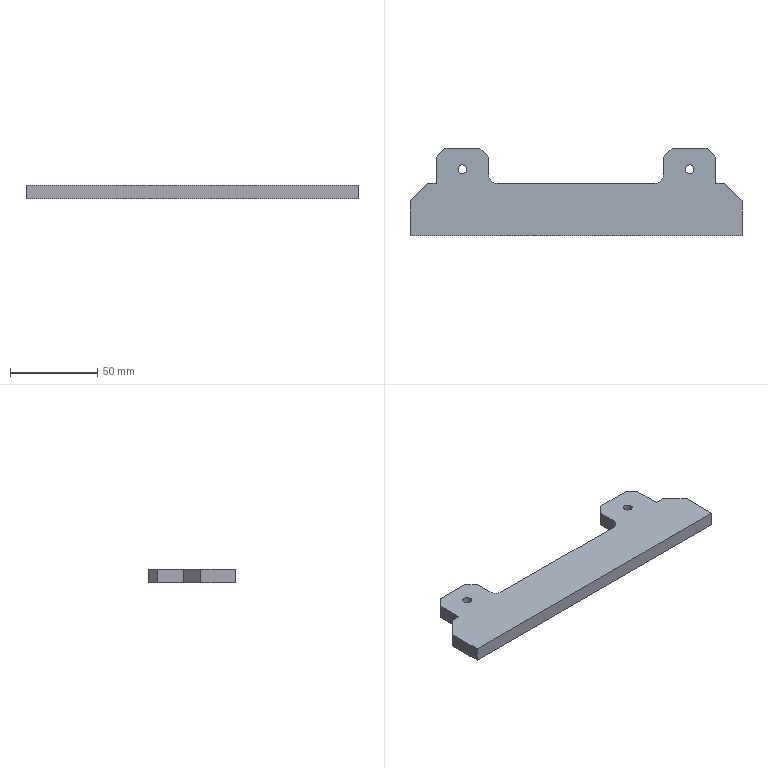Part | SolidWorks | features Chamfer 1, Extrusion 1, Fillet 1, HoleWzd 1, ICE 1 | 1 solid | 26 faces | box 190 x 50 x 8 mm | volume 53772 mm3 | plane 20 | cylinder 6 | commonest cylinder face diameters 5 x4 10 x2
STEP:
#1=CARTESIAN_POINT('',(-67.5,13.,0.));
#2=VERTEX_POINT('',#1);
#3=CARTESIAN_POINT('',(-62.5,13.,0.));
#4=VERTEX_POINT('',#3);
#5=CARTESIAN_POINT('',(-65.,13.,0.));
#6=DIRECTION('',(0.,0.,1.));
#7=DIRECTION('',(1.,0.,0.));
#8=AXIS2_PLACEMENT_3D('',#5,#6,#7);
#9=CIRCLE('',#8,2.5);
#10=EDGE_CURVE('',#2,#4,#9,.T.);
#11=ORIENTED_EDGE('',*,*,#10,.F.);
#12=CARTESIAN_POINT('',(-67.5,13.,8.));
#13=VERTEX_POINT('',#12);
#14=CARTESIAN_POINT('',(-67.5,13.,8.));
#15=DIRECTION('',(0.,0.,1.));
#16=VECTOR('',#15,1000.);
#17=LINE('',#14,#16);
#18=EDGE_CURVE('',#2,#13,#17,.T.);
#19=ORIENTED_EDGE('',*,*,#18,.T.);
#20=CARTESIAN_POINT('',(-62.5,13.,8.));
#21=VERTEX_POINT('',#20);
#22=CARTESIAN_POINT('',(-65.,13.,8.));
#23=DIRECTION('',(0.,0.,1.));
#24=DIRECTION('',(1.,0.,0.));
#25=AXIS2_PLACEMENT_3D('',#22,#23,#24);
#26=CIRCLE('',#25,2.5);
#27=EDGE_CURVE('',#13,#21,#26,.T.);
#28=ORIENTED_EDGE('',*,*,#27,.T.);
#29=CARTESIAN_POINT('',(-62.5,13.,8.));
#30=DIRECTION('',(0.,0.,1.));
#31=VECTOR('',#30,1000.);
#32=LINE('',#29,#31);
#33=EDGE_CURVE('',#4,#21,#32,.T.);
#34=ORIENTED_EDGE('',*,*,#33,.F.);
#35=EDGE_LOOP('',(#11,#19,#28,#34));
#36=FACE_OUTER_BOUND('',#35,.T.);
#37=CARTESIAN_POINT('',(-65.,13.,8.));
#38=DIRECTION('',(0.,0.,1.));
#39=DIRECTION('',(1.,0.,0.));
#40=AXIS2_PLACEMENT_3D('',#37,#38,#39);
#41=CYLINDRICAL_SURFACE('',#40,2.5);
#42=ADVANCED_FACE('',(#36),#41,.F.);
#43=CARTESIAN_POINT('',(62.5,13.,0.));
#44=VERTEX_POINT('',#43);
#45=CARTESIAN_POINT('',(67.5,13.,0.));
#46=VERTEX_POINT('',#45);
#47=CARTESIAN_POINT('',(65.,13.,0.));
#48=DIRECTION('',(0.,0.,1.));
#49=DIRECTION('',(1.,0.,0.));
#50=AXIS2_PLACEMENT_3D('',#47,#48,#49);
#51=CIRCLE('',#50,2.5);
#52=EDGE_CURVE('',#44,#46,#51,.T.);
#53=ORIENTED_EDGE('',*,*,#52,.F.);
#54=CARTESIAN_POINT('',(62.5,13.,8.));
#55=VERTEX_POINT('',#54);
#56=CARTESIAN_POINT('',(62.5,13.,8.));
#57=DIRECTION('',(0.,0.,1.));
#58=VECTOR('',#57,1000.);
#59=LINE('',#56,#58);
#60=EDGE_CURVE('',#44,#55,#59,.T.);
#61=ORIENTED_EDGE('',*,*,#60,.T.);
#62=CARTESIAN_POINT('',(67.5,13.,8.));
#63=VERTEX_POINT('',#62);
#64=CARTESIAN_POINT('',(65.,13.,8.));
#65=DIRECTION('',(0.,0.,1.));
#66=DIRECTION('',(1.,0.,0.));
#67=AXIS2_PLACEMENT_3D('',#64,#65,#66);
#68=CIRCLE('',#67,2.5);
#69=EDGE_CURVE('',#55,#63,#68,.T.);
#70=ORIENTED_EDGE('',*,*,#69,.T.);
#71=CARTESIAN_POINT('',(67.5,13.,8.));
#72=DIRECTION('',(0.,0.,1.));
#73=VECTOR('',#72,1000.);
#74=LINE('',#71,#73);
#75=EDGE_CURVE('',#46,#63,#74,.T.);
#76=ORIENTED_EDGE('',*,*,#75,.F.);
#77=EDGE_LOOP('',(#53,#61,#70,#76));
#78=FACE_OUTER_BOUND('',#77,.T.);
#79=CARTESIAN_POINT('',(65.,13.,8.));
#80=DIRECTION('',(0.,0.,1.));
#81=DIRECTION('',(1.,0.,0.));
#82=AXIS2_PLACEMENT_3D('',#79,#80,#81);
#83=CYLINDRICAL_SURFACE('',#82,2.5);
#84=ADVANCED_FACE('',(#78),#83,.F.);
#85=CARTESIAN_POINT('',(75.,25.,8.));
#86=VERTEX_POINT('',#85);
#87=CARTESIAN_POINT('',(55.,25.,8.));
#88=VERTEX_POINT('',#87);
#89=CARTESIAN_POINT('',(95.,25.,8.));
#90=DIRECTION('',(-1.,0.,0.));
#91=VECTOR('',#90,1000.);
#92=LINE('',#89,#91);
#93=EDGE_CURVE('',#86,#88,#92,.T.);
#94=ORIENTED_EDGE('',*,*,#93,.F.);
#95=CARTESIAN_POINT('',(75.,25.,0.));
#96=VERTEX_POINT('',#95);
#97=CARTESIAN_POINT('',(75.,25.,8.));
#98=DIRECTION('',(0.,0.,-1.));
#99=VECTOR('',#98,1000.);
#100=LINE('',#97,#99);
#101=EDGE_CURVE('',#86,#96,#100,.T.);
#102=ORIENTED_EDGE('',*,*,#101,.T.);
#103=CARTESIAN_POINT('',(55.,25.,0.));
#104=VERTEX_POINT('',#103);
#105=CARTESIAN_POINT('',(95.,25.,0.));
#106=DIRECTION('',(-1.,0.,0.));
#107=VECTOR('',#106,1000.);
#108=LINE('',#105,#107);
#109=EDGE_CURVE('',#96,#104,#108,.T.);
#110=ORIENTED_EDGE('',*,*,#109,.T.);
#111=CARTESIAN_POINT('',(55.,25.,8.));
#112=DIRECTION('',(0.,0.,1.));
#113=VECTOR('',#112,1000.);
#114=LINE('',#111,#113);
#115=EDGE_CURVE('',#104,#88,#114,.T.);
#116=ORIENTED_EDGE('',*,*,#115,.T.);
#117=EDGE_LOOP('',(#94,#102,#110,#116));
#118=FACE_OUTER_BOUND('',#117,.T.);
#119=CARTESIAN_POINT('',(95.,25.,8.));
#120=DIRECTION('',(0.,-1.,0.));
#121=DIRECTION('',(1.,0.,0.));
#122=AXIS2_PLACEMENT_3D('',#119,#120,#121);
#123=PLANE('',#122);
#124=ADVANCED_FACE('',(#118),#123,.F.);
#125=CARTESIAN_POINT('',(-95.,-5.,8.));
#126=VERTEX_POINT('',#125);
#127=CARTESIAN_POINT('',(-95.,-25.,8.));
#128=VERTEX_POINT('',#127);
#129=CARTESIAN_POINT('',(-95.,25.,8.));
#130=DIRECTION('',(0.,-1.,0.));
#131=VECTOR('',#130,1000.);
#132=LINE('',#129,#131);
#133=EDGE_CURVE('',#126,#128,#132,.T.);
#134=ORIENTED_EDGE('',*,*,#133,.F.);
#135=CARTESIAN_POINT('',(-95.,-5.,0.));
#136=VERTEX_POINT('',#135);
#137=CARTESIAN_POINT('',(-95.,-5.,0.));
#138=DIRECTION('',(0.,0.,1.));
#139=VECTOR('',#138,1000.);
#140=LINE('',#137,#139);
#141=EDGE_CURVE('',#136,#126,#140,.T.);
#142=ORIENTED_EDGE('',*,*,#141,.F.);
#143=CARTESIAN_POINT('',(-95.,-25.,0.));
#144=VERTEX_POINT('',#143);
#145=CARTESIAN_POINT('',(-95.,25.,0.));
#146=DIRECTION('',(0.,-1.,0.));
#147=VECTOR('',#146,1000.);
#148=LINE('',#145,#147);
#149=EDGE_CURVE('',#136,#144,#148,.T.);
#150=ORIENTED_EDGE('',*,*,#149,.T.);
#151=CARTESIAN_POINT('',(-95.,-25.,8.));
#152=DIRECTION('',(0.,0.,-1.));
#153=VECTOR('',#152,1000.);
#154=LINE('',#151,#153);
#155=EDGE_CURVE('',#128,#144,#154,.T.);
#156=ORIENTED_EDGE('',*,*,#155,.F.);
#157=EDGE_LOOP('',(#134,#142,#150,#156));
#158=FACE_OUTER_BOUND('',#157,.T.);
#159=CARTESIAN_POINT('',(-95.,25.,8.));
#160=DIRECTION('',(1.,0.,0.));
#161=DIRECTION('',(0.,1.,0.));
#162=AXIS2_PLACEMENT_3D('',#159,#160,#161);
#163=PLANE('',#162);
#164=ADVANCED_FACE('',(#158),#163,.F.);
#165=CARTESIAN_POINT('',(95.,-25.,0.));
#166=VERTEX_POINT('',#165);
#167=CARTESIAN_POINT('',(95.,-25.,0.));
#168=DIRECTION('',(1.,0.,0.));
#169=VECTOR('',#168,1000.);
#170=LINE('',#167,#169);
#171=EDGE_CURVE('',#144,#166,#170,.T.);
#172=ORIENTED_EDGE('',*,*,#171,.T.);
#173=CARTESIAN_POINT('',(95.,-25.,8.));
#174=VERTEX_POINT('',#173);
#175=CARTESIAN_POINT('',(95.,-25.,8.));
#176=DIRECTION('',(0.,0.,-1.));
#177=VECTOR('',#176,1000.);
#178=LINE('',#175,#177);
#179=EDGE_CURVE('',#174,#166,#178,.T.);
#180=ORIENTED_EDGE('',*,*,#179,.F.);
#181=CARTESIAN_POINT('',(95.,-25.,8.));
#182=DIRECTION('',(1.,0.,0.));
#183=VECTOR('',#182,1000.);
#184=LINE('',#181,#183);
#185=EDGE_CURVE('',#128,#174,#184,.T.);
#186=ORIENTED_EDGE('',*,*,#185,.F.);
#187=ORIENTED_EDGE('',*,*,#155,.T.);
#188=EDGE_LOOP('',(#172,#180,#186,#187));
#189=FACE_OUTER_BOUND('',#188,.T.);
#190=CARTESIAN_POINT('',(95.,-25.,8.));
#191=DIRECTION('',(0.,1.,0.));
#192=DIRECTION('',(-1.,0.,0.));
#193=AXIS2_PLACEMENT_3D('',#190,#191,#192);
#194=PLANE('',#193);
#195=ADVANCED_FACE('',(#189),#194,.F.);
#196=CARTESIAN_POINT('',(95.,-5.,0.));
#197=VERTEX_POINT('',#196);
#198=CARTESIAN_POINT('',(95.,25.,0.));
#199=DIRECTION('',(0.,1.,0.));
#200=VECTOR('',#199,1000.);
#201=LINE('',#198,#200);
#202=EDGE_CURVE('',#166,#197,#201,.T.);
#203=ORIENTED_EDGE('',*,*,#202,.T.);
#204=CARTESIAN_POINT('',(95.,-5.,8.));
#205=VERTEX_POINT('',#204);
#206=CARTESIAN_POINT('',(95.,-5.,0.));
#207=DIRECTION('',(0.,0.,1.));
#208=VECTOR('',#207,1000.);
#209=LINE('',#206,#208);
#210=EDGE_CURVE('',#197,#205,#209,.T.);
#211=ORIENTED_EDGE('',*,*,#210,.T.);
#212=CARTESIAN_POINT('',(95.,25.,8.));
#213=DIRECTION('',(0.,1.,0.));
#214=VECTOR('',#213,1000.);
#215=LINE('',#212,#214);
#216=EDGE_CURVE('',#174,#205,#215,.T.);
#217=ORIENTED_EDGE('',*,*,#216,.F.);
#218=ORIENTED_EDGE('',*,*,#179,.T.);
#219=EDGE_LOOP('',(#203,#211,#217,#218));
#220=FACE_OUTER_BOUND('',#219,.T.);
#221=CARTESIAN_POINT('',(95.,25.,8.));
#222=DIRECTION('',(-1.,0.,0.));
#223=DIRECTION('',(0.,0.,1.));
#224=AXIS2_PLACEMENT_3D('',#221,#222,#223);
#225=PLANE('',#224);
#226=ADVANCED_FACE('',(#220),#225,.F.);
#227=CARTESIAN_POINT('',(-55.,25.,8.));
#228=VERTEX_POINT('',#227);
#229=CARTESIAN_POINT('',(-75.,25.,8.));
#230=VERTEX_POINT('',#229);
#231=CARTESIAN_POINT('',(95.,25.,8.));
#232=DIRECTION('',(-1.,0.,0.));
#233=VECTOR('',#232,1000.);
#234=LINE('',#231,#233);
#235=EDGE_CURVE('',#228,#230,#234,.T.);
#236=ORIENTED_EDGE('',*,*,#235,.F.);
#237=CARTESIAN_POINT('',(-55.,25.,0.));
#238=VERTEX_POINT('',#237);
#239=CARTESIAN_POINT('',(-55.,25.,8.));
#240=DIRECTION('',(0.,0.,-1.));
#241=VECTOR('',#240,1000.);
#242=LINE('',#239,#241);
#243=EDGE_CURVE('',#228,#238,#242,.T.);
#244=ORIENTED_EDGE('',*,*,#243,.T.);
#245=CARTESIAN_POINT('',(-75.,25.,0.));
#246=VERTEX_POINT('',#245);
#247=CARTESIAN_POINT('',(95.,25.,0.));
#248=DIRECTION('',(-1.,0.,0.));
#249=VECTOR('',#248,1000.);
#250=LINE('',#247,#249);
#251=EDGE_CURVE('',#238,#246,#250,.T.);
#252=ORIENTED_EDGE('',*,*,#251,.T.);
#253=CARTESIAN_POINT('',(-75.,25.,8.));
#254=DIRECTION('',(0.,0.,1.));
#255=VECTOR('',#254,1000.);
#256=LINE('',#253,#255);
#257=EDGE_CURVE('',#246,#230,#256,.T.);
#258=ORIENTED_EDGE('',*,*,#257,.T.);
#259=EDGE_LOOP('',(#236,#244,#252,#258));
#260=FACE_OUTER_BOUND('',#259,.T.);
#261=CARTESIAN_POINT('',(95.,25.,8.));
#262=DIRECTION('',(0.,-1.,0.));
#263=DIRECTION('',(1.,0.,0.));
#264=AXIS2_PLACEMENT_3D('',#261,#262,#263);
#265=PLANE('',#264);
#266=ADVANCED_FACE('',(#260),#265,.F.);
#267=CARTESIAN_POINT('',(-65.,13.,8.));
#268=DIRECTION('',(0.,0.,1.));
#269=DIRECTION('',(1.,0.,0.));
#270=AXIS2_PLACEMENT_3D('',#267,#268,#269);
#271=CIRCLE('',#270,2.5);
#272=EDGE_CURVE('',#21,#13,#271,.T.);
#273=ORIENTED_EDGE('',*,*,#272,.F.);
#274=ORIENTED_EDGE('',*,*,#27,.F.);
#275=EDGE_LOOP('',(#273,#274));
#276=FACE_BOUND('',#275,.T.);
#277=CARTESIAN_POINT('',(65.,13.,8.));
#278=DIRECTION('',(0.,0.,1.));
#279=DIRECTION('',(1.,0.,0.));
#280=AXIS2_PLACEMENT_3D('',#277,#278,#279);
#281=CIRCLE('',#280,2.5);
#282=EDGE_CURVE('',#63,#55,#281,.T.);
#283=ORIENTED_EDGE('',*,*,#282,.F.);
#284=ORIENTED_EDGE('',*,*,#69,.F.);
#285=EDGE_LOOP('',(#283,#284));
#286=FACE_BOUND('',#285,.T.);
#287=CARTESIAN_POINT('',(80.,20.,8.));
#288=VERTEX_POINT('',#287);
#289=CARTESIAN_POINT('',(80.,5.,8.));
#290=VERTEX_POINT('',#289);
#291=CARTESIAN_POINT('',(80.,25.,8.));
#292=DIRECTION('',(0.,-1.,0.));
#293=VECTOR('',#292,1000.);
#294=LINE('',#291,#293);
#295=EDGE_CURVE('',#288,#290,#294,.T.);
#296=ORIENTED_EDGE('',*,*,#295,.F.);
#297=CARTESIAN_POINT('',(80.,20.,8.));
#298=DIRECTION('',(-0.7071,0.7071,0.));
#299=VECTOR('',#298,1000.);
#300=LINE('',#297,#299);
#301=EDGE_CURVE('',#288,#86,#300,.T.);
#302=ORIENTED_EDGE('',*,*,#301,.T.);
#303=ORIENTED_EDGE('',*,*,#93,.T.);
#304=CARTESIAN_POINT('',(50.,20.,8.));
#305=VERTEX_POINT('',#304);
#306=CARTESIAN_POINT('',(55.,25.,8.));
#307=DIRECTION('',(-0.7071,-0.7071,0.));
#308=VECTOR('',#307,1000.);
#309=LINE('',#306,#308);
#310=EDGE_CURVE('',#88,#305,#309,.T.);
#311=ORIENTED_EDGE('',*,*,#310,.T.);
#312=CARTESIAN_POINT('',(50.,10.,8.));
#313=VERTEX_POINT('',#312);
#314=CARTESIAN_POINT('',(50.,5.,8.));
#315=DIRECTION('',(0.,1.,0.));
#316=VECTOR('',#315,1000.);
#317=LINE('',#314,#316);
#318=EDGE_CURVE('',#313,#305,#317,.T.);
#319=ORIENTED_EDGE('',*,*,#318,.F.);
#320=CARTESIAN_POINT('',(45.,5.,8.));
#321=VERTEX_POINT('',#320);
#322=CARTESIAN_POINT('',(45.,10.,8.));
#323=DIRECTION('',(0.,0.,-1.));
#324=DIRECTION('',(-1.,0.,0.));
#325=AXIS2_PLACEMENT_3D('',#322,#323,#324);
#326=CIRCLE('',#325,5.);
#327=EDGE_CURVE('',#313,#321,#326,.T.);
#328=ORIENTED_EDGE('',*,*,#327,.T.);
#329=CARTESIAN_POINT('',(-45.,5.,8.));
#330=VERTEX_POINT('',#329);
#331=CARTESIAN_POINT('',(-50.,5.,8.));
#332=DIRECTION('',(1.,0.,0.));
#333=VECTOR('',#332,1000.);
#334=LINE('',#331,#333);
#335=EDGE_CURVE('',#330,#321,#334,.T.);
#336=ORIENTED_EDGE('',*,*,#335,.F.);
#337=CARTESIAN_POINT('',(-50.,10.,8.));
#338=VERTEX_POINT('',#337);
#339=CARTESIAN_POINT('',(-45.,10.,8.));
#340=DIRECTION('',(0.,0.,-1.));
#341=DIRECTION('',(-1.,0.,0.));
#342=AXIS2_PLACEMENT_3D('',#339,#340,#341);
#343=CIRCLE('',#342,5.);
#344=EDGE_CURVE('',#330,#338,#343,.T.);
#345=ORIENTED_EDGE('',*,*,#344,.T.);
#346=CARTESIAN_POINT('',(-50.,20.,8.));
#347=VERTEX_POINT('',#346);
#348=CARTESIAN_POINT('',(-50.,25.,8.));
#349=DIRECTION('',(0.,-1.,0.));
#350=VECTOR('',#349,1000.);
#351=LINE('',#348,#350);
#352=EDGE_CURVE('',#347,#338,#351,.T.);
#353=ORIENTED_EDGE('',*,*,#352,.F.);
#354=CARTESIAN_POINT('',(-50.,20.,8.));
#355=DIRECTION('',(-0.7071,0.7071,0.));
#356=VECTOR('',#355,1000.);
#357=LINE('',#354,#356);
#358=EDGE_CURVE('',#347,#228,#357,.T.);
#359=ORIENTED_EDGE('',*,*,#358,.T.);
#360=ORIENTED_EDGE('',*,*,#235,.T.);
#361=CARTESIAN_POINT('',(-80.,20.,8.));
#362=VERTEX_POINT('',#361);
#363=CARTESIAN_POINT('',(-75.,25.,8.));
#364=DIRECTION('',(-0.7071,-0.7071,0.));
#365=VECTOR('',#364,1000.);
#366=LINE('',#363,#365);
#367=EDGE_CURVE('',#230,#362,#366,.T.);
#368=ORIENTED_EDGE('',*,*,#367,.T.);
#369=CARTESIAN_POINT('',(-80.,5.,8.));
#370=VERTEX_POINT('',#369);
#371=CARTESIAN_POINT('',(-80.,5.,8.));
#372=DIRECTION('',(0.,1.,0.));
#373=VECTOR('',#372,1000.);
#374=LINE('',#371,#373);
#375=EDGE_CURVE('',#370,#362,#374,.T.);
#376=ORIENTED_EDGE('',*,*,#375,.F.);
#377=CARTESIAN_POINT('',(-85.,5.,8.));
#378=VERTEX_POINT('',#377);
#379=CARTESIAN_POINT('',(-85.,5.,8.));
#380=DIRECTION('',(1.,0.,0.));
#381=VECTOR('',#380,1000.);
#382=LINE('',#379,#381);
#383=EDGE_CURVE('',#378,#370,#382,.T.);
#384=ORIENTED_EDGE('',*,*,#383,.F.);
#385=CARTESIAN_POINT('',(-95.,-5.,8.));
#386=DIRECTION('',(0.7071,0.7071,0.));
#387=VECTOR('',#386,1000.);
#388=LINE('',#385,#387);
#389=EDGE_CURVE('',#126,#378,#388,.T.);
#390=ORIENTED_EDGE('',*,*,#389,.F.);
#391=ORIENTED_EDGE('',*,*,#133,.T.);
#392=ORIENTED_EDGE('',*,*,#185,.T.);
#393=ORIENTED_EDGE('',*,*,#216,.T.);
#394=CARTESIAN_POINT('',(85.,5.,8.));
#395=VERTEX_POINT('',#394);
#396=CARTESIAN_POINT('',(85.,5.,8.));
#397=DIRECTION('',(0.7071,-0.7071,0.));
#398=VECTOR('',#397,1000.);
#399=LINE('',#396,#398);
#400=EDGE_CURVE('',#395,#205,#399,.T.);
#401=ORIENTED_EDGE('',*,*,#400,.F.);
#402=CARTESIAN_POINT('',(80.,5.,8.));
#403=DIRECTION('',(1.,0.,0.));
#404=VECTOR('',#403,1000.);
#405=LINE('',#402,#404);
#406=EDGE_CURVE('',#290,#395,#405,.T.);
#407=ORIENTED_EDGE('',*,*,#406,.F.);
#408=EDGE_LOOP('',(#296,#302,#303,#311,#319,#328,#336,#345,#353,#359,#360,#368,#376,#384,#390,#391,#392,#393,#401,#407));
#409=FACE_OUTER_BOUND('',#408,.T.);
#410=CARTESIAN_POINT('',(0.,0.,8.));
#411=DIRECTION('',(0.,0.,-1.));
#412=DIRECTION('',(-1.,0.,0.));
#413=AXIS2_PLACEMENT_3D('',#410,#411,#412);
#414=PLANE('',#413);
#415=ADVANCED_FACE('',(#276,#286,#409),#414,.F.);
#416=CARTESIAN_POINT('',(-65.,13.,0.));
#417=DIRECTION('',(0.,0.,1.));
#418=DIRECTION('',(1.,0.,0.));
#419=AXIS2_PLACEMENT_3D('',#416,#417,#418);
#420=CIRCLE('',#419,2.5);
#421=EDGE_CURVE('',#4,#2,#420,.T.);
#422=ORIENTED_EDGE('',*,*,#421,.T.);
#423=ORIENTED_EDGE('',*,*,#10,.T.);
#424=EDGE_LOOP('',(#422,#423));
#425=FACE_BOUND('',#424,.T.);
#426=CARTESIAN_POINT('',(65.,13.,0.));
#427=DIRECTION('',(0.,0.,1.));
#428=DIRECTION('',(1.,0.,0.));
#429=AXIS2_PLACEMENT_3D('',#426,#427,#428);
#430=CIRCLE('',#429,2.5);
#431=EDGE_CURVE('',#46,#44,#430,.T.);
#432=ORIENTED_EDGE('',*,*,#431,.T.);
#433=ORIENTED_EDGE('',*,*,#52,.T.);
#434=EDGE_LOOP('',(#432,#433));
#435=FACE_BOUND('',#434,.T.);
#436=ORIENTED_EDGE('',*,*,#109,.F.);
#437=CARTESIAN_POINT('',(80.,20.,0.));
#438=VERTEX_POINT('',#437);
#439=CARTESIAN_POINT('',(50.,50.,0.));
#440=DIRECTION('',(0.7071,-0.7071,0.));
#441=VECTOR('',#440,1000.);
#442=LINE('',#439,#441);
#443=EDGE_CURVE('',#96,#438,#442,.T.);
#444=ORIENTED_EDGE('',*,*,#443,.T.);
#445=CARTESIAN_POINT('',(80.,5.,0.));
#446=VERTEX_POINT('',#445);
#447=CARTESIAN_POINT('',(80.,25.,0.));
#448=DIRECTION('',(0.,-1.,0.));
#449=VECTOR('',#448,1000.);
#450=LINE('',#447,#449);
#451=EDGE_CURVE('',#438,#446,#450,.T.);
#452=ORIENTED_EDGE('',*,*,#451,.T.);
#453=CARTESIAN_POINT('',(85.,5.,0.));
#454=VERTEX_POINT('',#453);
#455=CARTESIAN_POINT('',(80.,5.,0.));
#456=DIRECTION('',(1.,0.,0.));
#457=VECTOR('',#456,1000.);
#458=LINE('',#455,#457);
#459=EDGE_CURVE('',#446,#454,#458,.T.);
#460=ORIENTED_EDGE('',*,*,#459,.T.);
#461=CARTESIAN_POINT('',(85.,5.,0.));
#462=DIRECTION('',(0.7071,-0.7071,0.));
#463=VECTOR('',#462,1000.);
#464=LINE('',#461,#463);
#465=EDGE_CURVE('',#454,#197,#464,.T.);
#466=ORIENTED_EDGE('',*,*,#465,.T.);
#467=ORIENTED_EDGE('',*,*,#202,.F.);
#468=ORIENTED_EDGE('',*,*,#171,.F.);
#469=ORIENTED_EDGE('',*,*,#149,.F.);
#470=CARTESIAN_POINT('',(-85.,5.,0.));
#471=VERTEX_POINT('',#470);
#472=CARTESIAN_POINT('',(-95.,-5.,0.));
#473=DIRECTION('',(0.7071,0.7071,0.));
#474=VECTOR('',#473,1000.);
#475=LINE('',#472,#474);
#476=EDGE_CURVE('',#136,#471,#475,.T.);
#477=ORIENTED_EDGE('',*,*,#476,.T.);
#478=CARTESIAN_POINT('',(-80.,5.,0.));
#479=VERTEX_POINT('',#478);
#480=CARTESIAN_POINT('',(-85.,5.,0.));
#481=DIRECTION('',(1.,0.,0.));
#482=VECTOR('',#481,1000.);
#483=LINE('',#480,#482);
#484=EDGE_CURVE('',#471,#479,#483,.T.);
#485=ORIENTED_EDGE('',*,*,#484,.T.);
#486=CARTESIAN_POINT('',(-80.,20.,0.));
#487=VERTEX_POINT('',#486);
#488=CARTESIAN_POINT('',(-80.,5.,0.));
#489=DIRECTION('',(0.,1.,0.));
#490=VECTOR('',#489,1000.);
#491=LINE('',#488,#490);
#492=EDGE_CURVE('',#479,#487,#491,.T.);
#493=ORIENTED_EDGE('',*,*,#492,.T.);
#494=CARTESIAN_POINT('',(-50.,50.,0.));
#495=DIRECTION('',(0.7071,0.7071,0.));
#496=VECTOR('',#495,1000.);
#497=LINE('',#494,#496);
#498=EDGE_CURVE('',#487,#246,#497,.T.);
#499=ORIENTED_EDGE('',*,*,#498,.T.);
#500=ORIENTED_EDGE('',*,*,#251,.F.);
#501=CARTESIAN_POINT('',(-50.,20.,0.));
#502=VERTEX_POINT('',#501);
#503=CARTESIAN_POINT('',(-15.,-15.,0.));
#504=DIRECTION('',(0.7071,-0.7071,0.));
#505=VECTOR('',#504,1000.);
#506=LINE('',#503,#505);
#507=EDGE_CURVE('',#238,#502,#506,.T.);
#508=ORIENTED_EDGE('',*,*,#507,.T.);
#509=CARTESIAN_POINT('',(-50.,10.,0.));
#510=VERTEX_POINT('',#509);
#511=CARTESIAN_POINT('',(-50.,25.,0.));
#512=DIRECTION('',(0.,-1.,0.));
#513=VECTOR('',#512,1000.);
#514=LINE('',#511,#513);
#515=EDGE_CURVE('',#502,#510,#514,.T.);
#516=ORIENTED_EDGE('',*,*,#515,.T.);
#517=CARTESIAN_POINT('',(-45.,5.,0.));
#518=VERTEX_POINT('',#517);
#519=CARTESIAN_POINT('',(-45.,10.,0.));
#520=DIRECTION('',(0.,0.,1.));
#521=DIRECTION('',(-1.,0.,0.));
#522=AXIS2_PLACEMENT_3D('',#519,#520,#521);
#523=CIRCLE('',#522,5.);
#524=EDGE_CURVE('',#510,#518,#523,.T.);
#525=ORIENTED_EDGE('',*,*,#524,.T.);
#526=CARTESIAN_POINT('',(45.,5.,0.));
#527=VERTEX_POINT('',#526);
#528=CARTESIAN_POINT('',(-50.,5.,0.));
#529=DIRECTION('',(1.,0.,0.));
#530=VECTOR('',#529,1000.);
#531=LINE('',#528,#530);
#532=EDGE_CURVE('',#518,#527,#531,.T.);
#533=ORIENTED_EDGE('',*,*,#532,.T.);
#534=CARTESIAN_POINT('',(50.,10.,0.));
#535=VERTEX_POINT('',#534);
#536=CARTESIAN_POINT('',(45.,10.,0.));
#537=DIRECTION('',(0.,0.,1.));
#538=DIRECTION('',(-1.,0.,0.));
#539=AXIS2_PLACEMENT_3D('',#536,#537,#538);
#540=CIRCLE('',#539,5.);
#541=EDGE_CURVE('',#527,#535,#540,.T.);
#542=ORIENTED_EDGE('',*,*,#541,.T.);
#543=CARTESIAN_POINT('',(50.,20.,0.));
#544=VERTEX_POINT('',#543);
#545=CARTESIAN_POINT('',(50.,5.,0.));
#546=DIRECTION('',(0.,1.,0.));
#547=VECTOR('',#546,1000.);
#548=LINE('',#545,#547);
#549=EDGE_CURVE('',#535,#544,#548,.T.);
#550=ORIENTED_EDGE('',*,*,#549,.T.);
#551=CARTESIAN_POINT('',(15.,-15.,0.));
#552=DIRECTION('',(0.7071,0.7071,0.));
#553=VECTOR('',#552,1000.);
#554=LINE('',#551,#553);
#555=EDGE_CURVE('',#544,#104,#554,.T.);
#556=ORIENTED_EDGE('',*,*,#555,.T.);
#557=EDGE_LOOP('',(#436,#444,#452,#460,#466,#467,#468,#469,#477,#485,#493,#499,#500,#508,#516,#525,#533,#542,#550,#556));
#558=FACE_OUTER_BOUND('',#557,.T.);
#559=CARTESIAN_POINT('',(0.,0.,0.));
#560=DIRECTION('',(0.,0.,-1.));
#561=DIRECTION('',(-1.,0.,0.));
#562=AXIS2_PLACEMENT_3D('',#559,#560,#561);
#563=PLANE('',#562);
#564=ADVANCED_FACE('',(#425,#435,#558),#563,.T.);
#565=ORIENTED_EDGE('',*,*,#389,.T.);
#566=CARTESIAN_POINT('',(-85.,5.,0.));
#567=DIRECTION('',(0.,0.,1.));
#568=VECTOR('',#567,1000.);
#569=LINE('',#566,#568);
#570=EDGE_CURVE('',#471,#378,#569,.T.);
#571=ORIENTED_EDGE('',*,*,#570,.F.);
#572=ORIENTED_EDGE('',*,*,#476,.F.);
#573=ORIENTED_EDGE('',*,*,#141,.T.);
#574=EDGE_LOOP('',(#565,#571,#572,#573));
#575=FACE_OUTER_BOUND('',#574,.T.);
#576=CARTESIAN_POINT('',(-95.,-5.,0.));
#577=DIRECTION('',(0.7071,-0.7071,0.));
#578=DIRECTION('',(0.7071,0.7071,0.));
#579=AXIS2_PLACEMENT_3D('',#576,#577,#578);
#580=PLANE('',#579);
#581=ADVANCED_FACE('',(#575),#580,.F.);
#582=ORIENTED_EDGE('',*,*,#383,.T.);
#583=CARTESIAN_POINT('',(-80.,5.,0.));
#584=DIRECTION('',(0.,0.,1.));
#585=VECTOR('',#584,1000.);
#586=LINE('',#583,#585);
#587=EDGE_CURVE('',#479,#370,#586,.T.);
#588=ORIENTED_EDGE('',*,*,#587,.F.);
#589=ORIENTED_EDGE('',*,*,#484,.F.);
#590=ORIENTED_EDGE('',*,*,#570,.T.);
#591=EDGE_LOOP('',(#582,#588,#589,#590));
#592=FACE_OUTER_BOUND('',#591,.T.);
#593=CARTESIAN_POINT('',(-85.,5.,0.));
#594=DIRECTION('',(0.,-1.,0.));
#595=DIRECTION('',(0.,0.,-1.));
#596=AXIS2_PLACEMENT_3D('',#593,#594,#595);
#597=PLANE('',#596);
#598=ADVANCED_FACE('',(#592),#597,.F.);
#599=ORIENTED_EDGE('',*,*,#375,.T.);
#600=CARTESIAN_POINT('',(-80.,20.,0.));
#601=DIRECTION('',(0.,0.,-1.));
#602=VECTOR('',#601,1000.);
#603=LINE('',#600,#602);
#604=EDGE_CURVE('',#362,#487,#603,.T.);
#605=ORIENTED_EDGE('',*,*,#604,.T.);
#606=ORIENTED_EDGE('',*,*,#492,.F.);
#607=ORIENTED_EDGE('',*,*,#587,.T.);
#608=EDGE_LOOP('',(#599,#605,#606,#607));
#609=FACE_OUTER_BOUND('',#608,.T.);
#610=CARTESIAN_POINT('',(-80.,5.,0.));
#611=DIRECTION('',(1.,0.,0.));
#612=DIRECTION('',(0.,0.,-1.));
#613=AXIS2_PLACEMENT_3D('',#610,#611,#612);
#614=PLANE('',#613);
#615=ADVANCED_FACE('',(#609),#614,.F.);
#616=ORIENTED_EDGE('',*,*,#352,.T.);
#617=CARTESIAN_POINT('',(-50.,10.,0.));
#618=DIRECTION('',(0.,0.,-1.));
#619=VECTOR('',#618,1000.);
#620=LINE('',#617,#619);
#621=EDGE_CURVE('',#338,#510,#620,.T.);
#622=ORIENTED_EDGE('',*,*,#621,.T.);
#623=ORIENTED_EDGE('',*,*,#515,.F.);
#624=CARTESIAN_POINT('',(-50.,20.,0.));
#625=DIRECTION('',(0.,0.,1.));
#626=VECTOR('',#625,1000.);
#627=LINE('',#624,#626);
#628=EDGE_CURVE('',#502,#347,#627,.T.);
#629=ORIENTED_EDGE('',*,*,#628,.T.);
#630=EDGE_LOOP('',(#616,#622,#623,#629));
#631=FACE_OUTER_BOUND('',#630,.T.);
#632=CARTESIAN_POINT('',(-50.,25.,0.));
#633=DIRECTION('',(-1.,0.,0.));
#634=DIRECTION('',(0.,-1.,0.));
#635=AXIS2_PLACEMENT_3D('',#632,#633,#634);
#636=PLANE('',#635);
#637=ADVANCED_FACE('',(#631),#636,.F.);
#638=ORIENTED_EDGE('',*,*,#335,.T.);
#639=CARTESIAN_POINT('',(45.,5.,0.));
#640=DIRECTION('',(0.,0.,-1.));
#641=VECTOR('',#640,1000.);
#642=LINE('',#639,#641);
#643=EDGE_CURVE('',#321,#527,#642,.T.);
#644=ORIENTED_EDGE('',*,*,#643,.T.);
#645=ORIENTED_EDGE('',*,*,#532,.F.);
#646=CARTESIAN_POINT('',(-45.,5.,8.));
#647=DIRECTION('',(0.,0.,1.));
#648=VECTOR('',#647,1000.);
#649=LINE('',#646,#648);
#650=EDGE_CURVE('',#518,#330,#649,.T.);
#651=ORIENTED_EDGE('',*,*,#650,.T.);
#652=EDGE_LOOP('',(#638,#644,#645,#651));
#653=FACE_OUTER_BOUND('',#652,.T.);
#654=CARTESIAN_POINT('',(-50.,5.,0.));
#655=DIRECTION('',(0.,-1.,0.));
#656=DIRECTION('',(0.,0.,-1.));
#657=AXIS2_PLACEMENT_3D('',#654,#655,#656);
#658=PLANE('',#657);
#659=ADVANCED_FACE('',(#653),#658,.F.);
#660=ORIENTED_EDGE('',*,*,#549,.F.);
#661=CARTESIAN_POINT('',(50.,10.,8.));
#662=DIRECTION('',(0.,0.,1.));
#663=VECTOR('',#662,1000.);
#664=LINE('',#661,#663);
#665=EDGE_CURVE('',#535,#313,#664,.T.);
#666=ORIENTED_EDGE('',*,*,#665,.T.);
#667=ORIENTED_EDGE('',*,*,#318,.T.);
#668=CARTESIAN_POINT('',(50.,20.,0.));
#669=DIRECTION('',(0.,0.,-1.));
#670=VECTOR('',#669,1000.);
#671=LINE('',#668,#670);
#672=EDGE_CURVE('',#305,#544,#671,.T.);
#673=ORIENTED_EDGE('',*,*,#672,.T.);
#674=EDGE_LOOP('',(#660,#666,#667,#673));
#675=FACE_OUTER_BOUND('',#674,.T.);
#676=CARTESIAN_POINT('',(50.,5.,0.));
#677=DIRECTION('',(1.,0.,0.));
#678=DIRECTION('',(0.,1.,0.));
#679=AXIS2_PLACEMENT_3D('',#676,#677,#678);
#680=PLANE('',#679);
#681=ADVANCED_FACE('',(#675),#680,.F.);
#682=ORIENTED_EDGE('',*,*,#400,.T.);
#683=ORIENTED_EDGE('',*,*,#210,.F.);
#684=ORIENTED_EDGE('',*,*,#465,.F.);
#685=CARTESIAN_POINT('',(85.,5.,0.));
#686=DIRECTION('',(0.,0.,1.));
#687=VECTOR('',#686,1000.);
#688=LINE('',#685,#687);
#689=EDGE_CURVE('',#454,#395,#688,.T.);
#690=ORIENTED_EDGE('',*,*,#689,.T.);
#691=EDGE_LOOP('',(#682,#683,#684,#690));
#692=FACE_OUTER_BOUND('',#691,.T.);
#693=CARTESIAN_POINT('',(85.,5.,0.));
#694=DIRECTION('',(-0.7071,-0.7071,0.));
#695=DIRECTION('',(0.7071,-0.7071,0.));
#696=AXIS2_PLACEMENT_3D('',#693,#694,#695);
#697=PLANE('',#696);
#698=ADVANCED_FACE('',(#692),#697,.F.);
#699=ORIENTED_EDGE('',*,*,#406,.T.);
#700=ORIENTED_EDGE('',*,*,#689,.F.);
#701=ORIENTED_EDGE('',*,*,#459,.F.);
#702=CARTESIAN_POINT('',(80.,5.,0.));
#703=DIRECTION('',(0.,0.,1.));
#704=VECTOR('',#703,1000.);
#705=LINE('',#702,#704);
#706=EDGE_CURVE('',#446,#290,#705,.T.);
#707=ORIENTED_EDGE('',*,*,#706,.T.);
#708=EDGE_LOOP('',(#699,#700,#701,#707));
#709=FACE_OUTER_BOUND('',#708,.T.);
#710=CARTESIAN_POINT('',(80.,5.,0.));
#711=DIRECTION('',(0.,-1.,0.));
#712=DIRECTION('',(0.,0.,-1.));
#713=AXIS2_PLACEMENT_3D('',#710,#711,#712);
#714=PLANE('',#713);
#715=ADVANCED_FACE('',(#709),#714,.F.);
#716=ORIENTED_EDGE('',*,*,#451,.F.);
#717=CARTESIAN_POINT('',(80.,20.,0.));
#718=DIRECTION('',(0.,0.,1.));
#719=VECTOR('',#718,1000.);
#720=LINE('',#717,#719);
#721=EDGE_CURVE('',#438,#288,#720,.T.);
#722=ORIENTED_EDGE('',*,*,#721,.T.);
#723=ORIENTED_EDGE('',*,*,#295,.T.);
#724=ORIENTED_EDGE('',*,*,#706,.F.);
#725=EDGE_LOOP('',(#716,#722,#723,#724));
#726=FACE_OUTER_BOUND('',#725,.T.);
#727=CARTESIAN_POINT('',(80.,25.,0.));
#728=DIRECTION('',(-1.,0.,0.));
#729=DIRECTION('',(0.,-1.,0.));
#730=AXIS2_PLACEMENT_3D('',#727,#728,#729);
#731=PLANE('',#730);
#732=ADVANCED_FACE('',(#726),#731,.F.);
#733=ORIENTED_EDGE('',*,*,#443,.F.);
#734=ORIENTED_EDGE('',*,*,#101,.F.);
#735=ORIENTED_EDGE('',*,*,#301,.F.);
#736=ORIENTED_EDGE('',*,*,#721,.F.);
#737=EDGE_LOOP('',(#733,#734,#735,#736));
#738=FACE_OUTER_BOUND('',#737,.T.);
#739=CARTESIAN_POINT('',(80.,20.,0.));
#740=DIRECTION('',(-0.7071,-0.7071,0.));
#741=DIRECTION('',(0.,0.,1.));
#742=AXIS2_PLACEMENT_3D('',#739,#740,#741);
#743=PLANE('',#742);
#744=ADVANCED_FACE('',(#738),#743,.F.);
#745=ORIENTED_EDGE('',*,*,#507,.F.);
#746=ORIENTED_EDGE('',*,*,#243,.F.);
#747=ORIENTED_EDGE('',*,*,#358,.F.);
#748=ORIENTED_EDGE('',*,*,#628,.F.);
#749=EDGE_LOOP('',(#745,#746,#747,#748));
#750=FACE_OUTER_BOUND('',#749,.T.);
#751=CARTESIAN_POINT('',(-50.,20.,0.));
#752=DIRECTION('',(-0.7071,-0.7071,0.));
#753=DIRECTION('',(0.,0.,1.));
#754=AXIS2_PLACEMENT_3D('',#751,#752,#753);
#755=PLANE('',#754);
#756=ADVANCED_FACE('',(#750),#755,.F.);
#757=ORIENTED_EDGE('',*,*,#555,.F.);
#758=ORIENTED_EDGE('',*,*,#672,.F.);
#759=ORIENTED_EDGE('',*,*,#310,.F.);
#760=ORIENTED_EDGE('',*,*,#115,.F.);
#761=EDGE_LOOP('',(#757,#758,#759,#760));
#762=FACE_OUTER_BOUND('',#761,.T.);
#763=CARTESIAN_POINT('',(55.,25.,8.));
#764=DIRECTION('',(0.7071,-0.7071,0.));
#765=DIRECTION('',(0.,0.,1.));
#766=AXIS2_PLACEMENT_3D('',#763,#764,#765);
#767=PLANE('',#766);
#768=ADVANCED_FACE('',(#762),#767,.F.);
#769=ORIENTED_EDGE('',*,*,#498,.F.);
#770=ORIENTED_EDGE('',*,*,#604,.F.);
#771=ORIENTED_EDGE('',*,*,#367,.F.);
#772=ORIENTED_EDGE('',*,*,#257,.F.);
#773=EDGE_LOOP('',(#769,#770,#771,#772));
#774=FACE_OUTER_BOUND('',#773,.T.);
#775=CARTESIAN_POINT('',(-75.,25.,8.));
#776=DIRECTION('',(0.7071,-0.7071,0.));
#777=DIRECTION('',(0.,0.,1.));
#778=AXIS2_PLACEMENT_3D('',#775,#776,#777);
#779=PLANE('',#778);
#780=ADVANCED_FACE('',(#774),#779,.F.);
#781=ORIENTED_EDGE('',*,*,#60,.F.);
#782=ORIENTED_EDGE('',*,*,#431,.F.);
#783=ORIENTED_EDGE('',*,*,#75,.T.);
#784=ORIENTED_EDGE('',*,*,#282,.T.);
#785=EDGE_LOOP('',(#781,#782,#783,#784));
#786=FACE_OUTER_BOUND('',#785,.T.);
#787=CARTESIAN_POINT('',(65.,13.,8.));
#788=DIRECTION('',(0.,0.,1.));
#789=DIRECTION('',(1.,0.,0.));
#790=AXIS2_PLACEMENT_3D('',#787,#788,#789);
#791=CYLINDRICAL_SURFACE('',#790,2.5);
#792=ADVANCED_FACE('',(#786),#791,.F.);
#793=ORIENTED_EDGE('',*,*,#18,.F.);
#794=ORIENTED_EDGE('',*,*,#421,.F.);
#795=ORIENTED_EDGE('',*,*,#33,.T.);
#796=ORIENTED_EDGE('',*,*,#272,.T.);
#797=EDGE_LOOP('',(#793,#794,#795,#796));
#798=FACE_OUTER_BOUND('',#797,.T.);
#799=CARTESIAN_POINT('',(-65.,13.,8.));
#800=DIRECTION('',(0.,0.,1.));
#801=DIRECTION('',(1.,0.,0.));
#802=AXIS2_PLACEMENT_3D('',#799,#800,#801);
#803=CYLINDRICAL_SURFACE('',#802,2.5);
#804=ADVANCED_FACE('',(#798),#803,.F.);
#805=ORIENTED_EDGE('',*,*,#541,.F.);
#806=ORIENTED_EDGE('',*,*,#643,.F.);
#807=ORIENTED_EDGE('',*,*,#327,.F.);
#808=ORIENTED_EDGE('',*,*,#665,.F.);
#809=EDGE_LOOP('',(#805,#806,#807,#808));
#810=FACE_OUTER_BOUND('',#809,.T.);
#811=CARTESIAN_POINT('',(45.,10.,0.));
#812=DIRECTION('',(0.,0.,-1.));
#813=DIRECTION('',(-1.,0.,0.));
#814=AXIS2_PLACEMENT_3D('',#811,#812,#813);
#815=CYLINDRICAL_SURFACE('',#814,5.);
#816=ADVANCED_FACE('',(#810),#815,.F.);
#817=ORIENTED_EDGE('',*,*,#524,.F.);
#818=ORIENTED_EDGE('',*,*,#621,.F.);
#819=ORIENTED_EDGE('',*,*,#344,.F.);
#820=ORIENTED_EDGE('',*,*,#650,.F.);
#821=EDGE_LOOP('',(#817,#818,#819,#820));
#822=FACE_OUTER_BOUND('',#821,.T.);
#823=CARTESIAN_POINT('',(-45.,10.,0.));
#824=DIRECTION('',(0.,0.,-1.));
#825=DIRECTION('',(-1.,0.,0.));
#826=AXIS2_PLACEMENT_3D('',#823,#824,#825);
#827=CYLINDRICAL_SURFACE('',#826,5.);
#828=ADVANCED_FACE('',(#822),#827,.F.);
#829=CLOSED_SHELL('',(#42,#84,#124,#164,#195,#226,#266,#415,#564,#581,#598,#615,#637,#659,#681,#698,#715,#732,#744,#756,#768,#780,#792,#804,#816,#828));
#830=MANIFOLD_SOLID_BREP('',#829);
#831=CARTESIAN_POINT('',(0.,0.,0.));
#832=DIRECTION('',(0.,0.,1.));
#833=DIRECTION('',(1.,0.,0.));
#834=AXIS2_PLACEMENT_3D('',#831,#832,#833);
#835=(LENGTH_UNIT()NAMED_UNIT(*)SI_UNIT(.MILLI.,.METRE.));
#836=UNCERTAINTY_MEASURE_WITH_UNIT(LENGTH_MEASURE(0.00001),#835,'','');
#837=(NAMED_UNIT(*)PLANE_ANGLE_UNIT()SI_UNIT($,.RADIAN.));
#838=(NAMED_UNIT(*)SI_UNIT($,.STERADIAN.)SOLID_ANGLE_UNIT());
#839=(GEOMETRIC_REPRESENTATION_CONTEXT(3)GLOBAL_UNCERTAINTY_ASSIGNED_CONTEXT((#836))GLOBAL_UNIT_ASSIGNED_CONTEXT((#835,#837,#838))REPRESENTATION_CONTEXT('',''));
#840=ADVANCED_BREP_SHAPE_REPRESENTATION('',(#830,#834),#839);